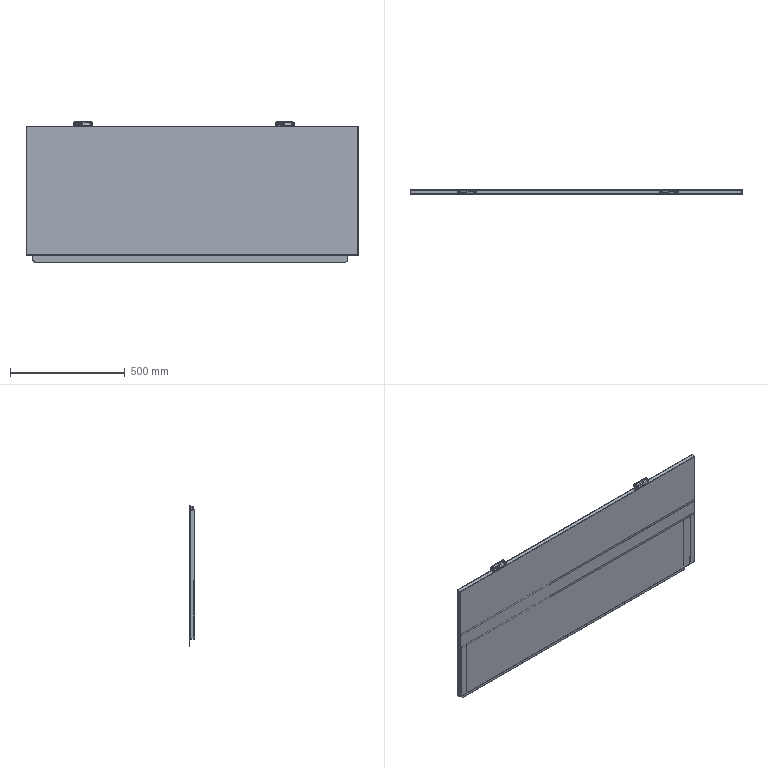Part | SolidWorks | 8 solids | 358 faces | box 1445 x 21.5 x 610.75 mm | volume 1744268 mm3 | plane 212 | cylinder 126 | cone 16 | spline 4 | commonest cylinder face diameters 3.3 x24 0.4 x20 3.4 x20 4.2 x16 8 x14 14.5 x12